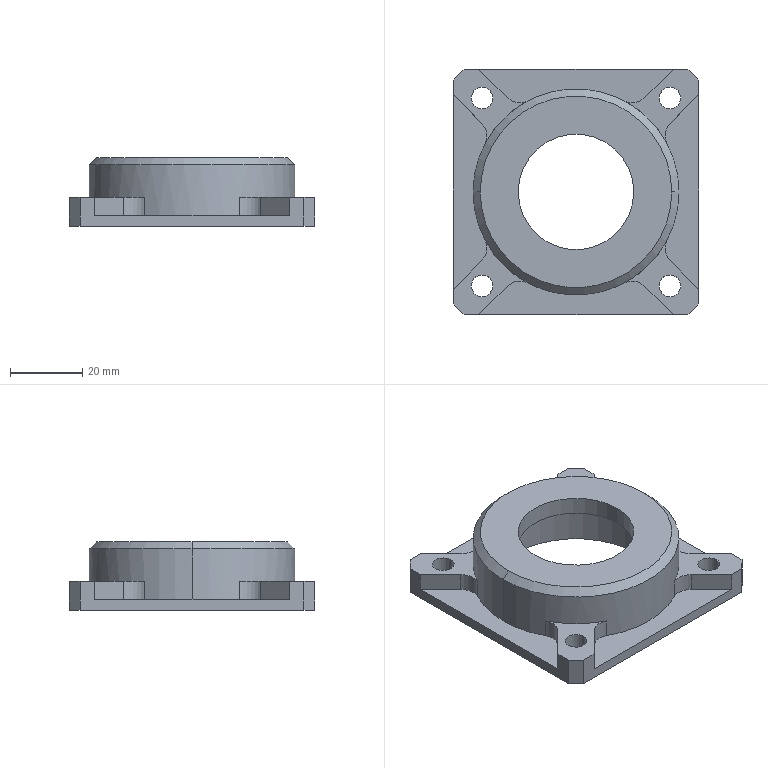Part | STEP file | Bearing seat | 1 solid | 53 faces | box 68 x 68 x 19 mm | volume 28550 mm3 | plane 27 | cylinder 24 | cone 2 | commonest cylinder face diameters 10 x10 6 x8 32 x2 47 x2 57 x2